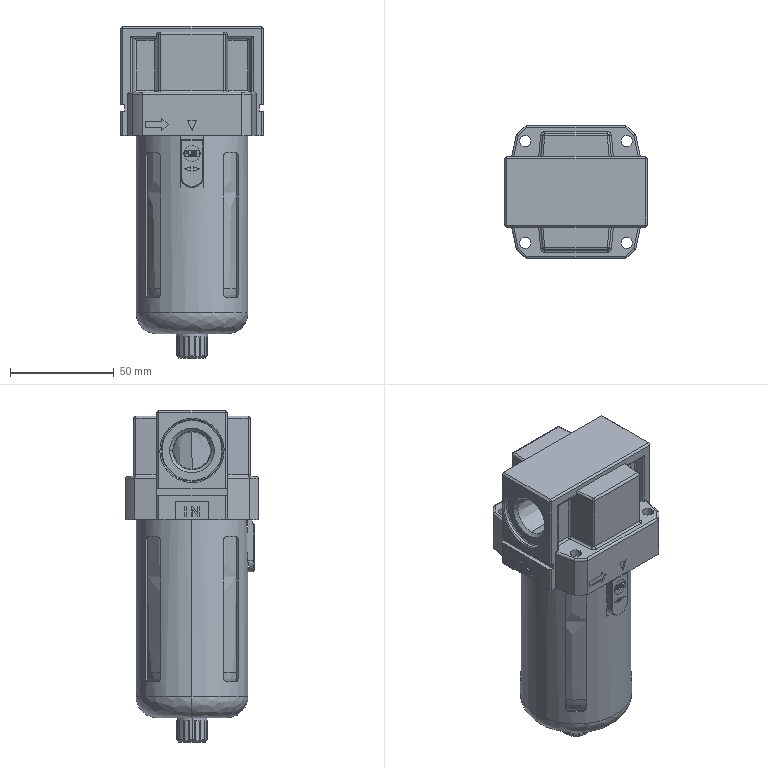Part | SolidWorks | features BaseBody 2 | 2 solids | 723 faces | box 68.8 x 64 x 160 mm | volume 171745 mm3 | plane 407 | cylinder 190 | spline 56 | cone 46 | torus 22 | sphere 2 | commonest cylinder face diameters 2 x64 4 x16 5.5 x8 14.3 x8 63.8 x8 59 x7